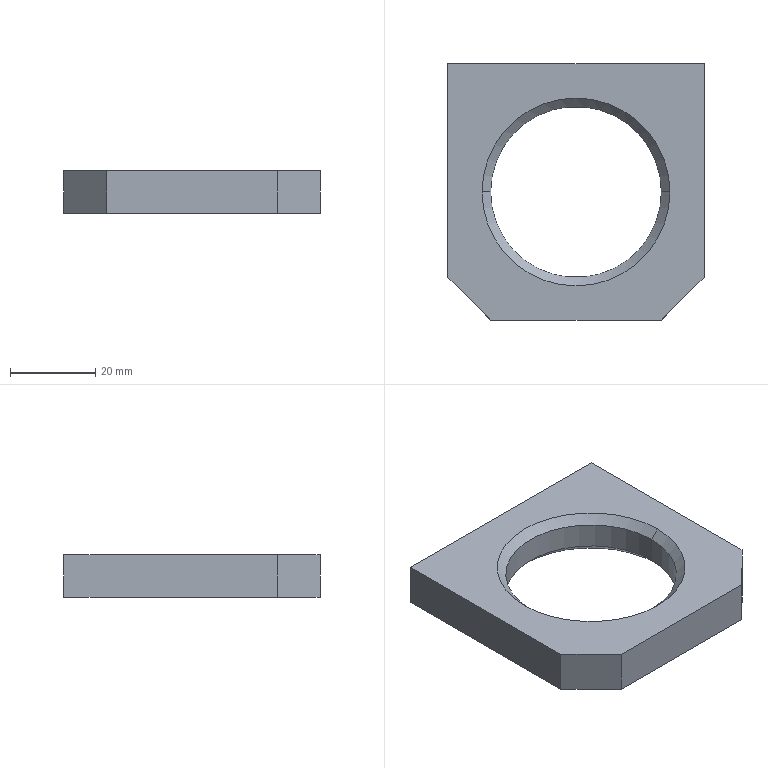Part | SolidWorks | features Chamfer 2, Extrusion 1 | 1 solid | 14 faces | box 60 x 60 x 10 mm | volume 21914 mm3 | plane 8 | cone 4 | cylinder 2 | commonest cylinder face diameters 40 x2
STEP:
#1=CARTESIAN_POINT('',(-20.,0.,8.));
#2=VERTEX_POINT('',#1);
#3=CARTESIAN_POINT('',(20.,0.,8.));
#4=VERTEX_POINT('',#3);
#5=CARTESIAN_POINT('',(0.,0.,8.));
#6=DIRECTION('',(0.,0.,1.));
#7=DIRECTION('',(-1.,0.,0.));
#8=AXIS2_PLACEMENT_3D('',#5,#6,#7);
#9=CIRCLE('',#8,20.);
#10=EDGE_CURVE('',#2,#4,#9,.T.);
#11=ORIENTED_EDGE('',*,*,#10,.F.);
#12=CARTESIAN_POINT('',(-22.,0.,10.));
#13=VERTEX_POINT('',#12);
#14=CARTESIAN_POINT('',(-20.,0.,8.));
#15=DIRECTION('',(-0.7071,0.,0.7071));
#16=VECTOR('',#15,1000.);
#17=LINE('',#14,#16);
#18=EDGE_CURVE('',#2,#13,#17,.T.);
#19=ORIENTED_EDGE('',*,*,#18,.T.);
#20=CARTESIAN_POINT('',(22.,0.,10.));
#21=VERTEX_POINT('',#20);
#22=CARTESIAN_POINT('',(0.,0.,10.));
#23=DIRECTION('',(0.,0.,-1.));
#24=DIRECTION('',(-1.,0.,0.));
#25=AXIS2_PLACEMENT_3D('',#22,#23,#24);
#26=CIRCLE('',#25,22.);
#27=EDGE_CURVE('',#21,#13,#26,.T.);
#28=ORIENTED_EDGE('',*,*,#27,.F.);
#29=CARTESIAN_POINT('',(20.,0.,8.));
#30=DIRECTION('',(0.7071,0.,0.7071));
#31=VECTOR('',#30,1000.);
#32=LINE('',#29,#31);
#33=EDGE_CURVE('',#4,#21,#32,.T.);
#34=ORIENTED_EDGE('',*,*,#33,.F.);
#35=EDGE_LOOP('',(#11,#19,#28,#34));
#36=FACE_OUTER_BOUND('',#35,.T.);
#37=CARTESIAN_POINT('',(0.,0.,8.));
#38=DIRECTION('',(0.,0.,1.));
#39=DIRECTION('',(1.,0.,0.));
#40=AXIS2_PLACEMENT_3D('',#37,#38,#39);
#41=CONICAL_SURFACE('',#40,20.,0.7854);
#42=ADVANCED_FACE('',(#36),#41,.F.);
#43=CARTESIAN_POINT('',(20.,0.,2.));
#44=VERTEX_POINT('',#43);
#45=CARTESIAN_POINT('',(-20.,0.,2.));
#46=VERTEX_POINT('',#45);
#47=CARTESIAN_POINT('',(0.,0.,2.));
#48=DIRECTION('',(0.,0.,-1.));
#49=DIRECTION('',(-1.,0.,0.));
#50=AXIS2_PLACEMENT_3D('',#47,#48,#49);
#51=CIRCLE('',#50,20.);
#52=EDGE_CURVE('',#44,#46,#51,.T.);
#53=ORIENTED_EDGE('',*,*,#52,.F.);
#54=CARTESIAN_POINT('',(22.,0.,0.));
#55=VERTEX_POINT('',#54);
#56=CARTESIAN_POINT('',(22.,0.,0.));
#57=DIRECTION('',(0.7071,0.,-0.7071));
#58=VECTOR('',#57,1000.);
#59=LINE('',#56,#58);
#60=EDGE_CURVE('',#44,#55,#59,.T.);
#61=ORIENTED_EDGE('',*,*,#60,.T.);
#62=CARTESIAN_POINT('',(-22.,0.,0.));
#63=VERTEX_POINT('',#62);
#64=CARTESIAN_POINT('',(0.,0.,0.));
#65=DIRECTION('',(0.,0.,1.));
#66=DIRECTION('',(-1.,0.,0.));
#67=AXIS2_PLACEMENT_3D('',#64,#65,#66);
#68=CIRCLE('',#67,22.);
#69=EDGE_CURVE('',#63,#55,#68,.T.);
#70=ORIENTED_EDGE('',*,*,#69,.F.);
#71=CARTESIAN_POINT('',(-22.,0.,0.));
#72=DIRECTION('',(-0.7071,0.,-0.7071));
#73=VECTOR('',#72,1000.);
#74=LINE('',#71,#73);
#75=EDGE_CURVE('',#46,#63,#74,.T.);
#76=ORIENTED_EDGE('',*,*,#75,.F.);
#77=EDGE_LOOP('',(#53,#61,#70,#76));
#78=FACE_OUTER_BOUND('',#77,.T.);
#79=CARTESIAN_POINT('',(0.,0.,0.));
#80=DIRECTION('',(0.,0.,-1.));
#81=DIRECTION('',(-1.,0.,0.));
#82=AXIS2_PLACEMENT_3D('',#79,#80,#81);
#83=CONICAL_SURFACE('',#82,22.,0.7854);
#84=ADVANCED_FACE('',(#78),#83,.F.);
#85=ORIENTED_EDGE('',*,*,#10,.T.);
#86=CARTESIAN_POINT('',(20.,0.,10.));
#87=DIRECTION('',(0.,0.,-1.));
#88=VECTOR('',#87,1000.);
#89=LINE('',#86,#88);
#90=EDGE_CURVE('',#4,#44,#89,.T.);
#91=ORIENTED_EDGE('',*,*,#90,.T.);
#92=ORIENTED_EDGE('',*,*,#52,.T.);
#93=CARTESIAN_POINT('',(-20.,0.,10.));
#94=DIRECTION('',(0.,0.,-1.));
#95=VECTOR('',#94,1000.);
#96=LINE('',#93,#95);
#97=EDGE_CURVE('',#2,#46,#96,.T.);
#98=ORIENTED_EDGE('',*,*,#97,.F.);
#99=EDGE_LOOP('',(#85,#91,#92,#98));
#100=FACE_OUTER_BOUND('',#99,.T.);
#101=CARTESIAN_POINT('',(0.,0.,10.));
#102=DIRECTION('',(0.,0.,-1.));
#103=DIRECTION('',(-1.,0.,0.));
#104=AXIS2_PLACEMENT_3D('',#101,#102,#103);
#105=CYLINDRICAL_SURFACE('',#104,20.);
#106=ADVANCED_FACE('',(#100),#105,.F.);
#107=ORIENTED_EDGE('',*,*,#27,.T.);
#108=CARTESIAN_POINT('',(0.,0.,10.));
#109=DIRECTION('',(0.,0.,-1.));
#110=DIRECTION('',(-1.,0.,0.));
#111=AXIS2_PLACEMENT_3D('',#108,#109,#110);
#112=CIRCLE('',#111,22.);
#113=EDGE_CURVE('',#13,#21,#112,.T.);
#114=ORIENTED_EDGE('',*,*,#113,.T.);
#115=EDGE_LOOP('',(#107,#114));
#116=FACE_BOUND('',#115,.T.);
#117=CARTESIAN_POINT('',(-20.,-30.,10.));
#118=VERTEX_POINT('',#117);
#119=CARTESIAN_POINT('',(20.,-30.,10.));
#120=VERTEX_POINT('',#119);
#121=CARTESIAN_POINT('',(-30.,-30.,10.));
#122=DIRECTION('',(1.,0.,0.));
#123=VECTOR('',#122,1000.);
#124=LINE('',#121,#123);
#125=EDGE_CURVE('',#118,#120,#124,.T.);
#126=ORIENTED_EDGE('',*,*,#125,.T.);
#127=CARTESIAN_POINT('',(30.,-20.,10.));
#128=VERTEX_POINT('',#127);
#129=CARTESIAN_POINT('',(30.,-20.,10.));
#130=DIRECTION('',(0.7071,0.7071,0.));
#131=VECTOR('',#130,1000.);
#132=LINE('',#129,#131);
#133=EDGE_CURVE('',#120,#128,#132,.T.);
#134=ORIENTED_EDGE('',*,*,#133,.T.);
#135=CARTESIAN_POINT('',(30.,30.,10.));
#136=VERTEX_POINT('',#135);
#137=CARTESIAN_POINT('',(30.,-30.,10.));
#138=DIRECTION('',(0.,1.,0.));
#139=VECTOR('',#138,1000.);
#140=LINE('',#137,#139);
#141=EDGE_CURVE('',#128,#136,#140,.T.);
#142=ORIENTED_EDGE('',*,*,#141,.T.);
#143=CARTESIAN_POINT('',(-30.,30.,10.));
#144=VERTEX_POINT('',#143);
#145=CARTESIAN_POINT('',(-30.,30.,10.));
#146=DIRECTION('',(-1.,0.,0.));
#147=VECTOR('',#146,1000.);
#148=LINE('',#145,#147);
#149=EDGE_CURVE('',#136,#144,#148,.T.);
#150=ORIENTED_EDGE('',*,*,#149,.T.);
#151=CARTESIAN_POINT('',(-30.,-20.,10.));
#152=VERTEX_POINT('',#151);
#153=CARTESIAN_POINT('',(-30.,-30.,10.));
#154=DIRECTION('',(0.,-1.,0.));
#155=VECTOR('',#154,1000.);
#156=LINE('',#153,#155);
#157=EDGE_CURVE('',#144,#152,#156,.T.);
#158=ORIENTED_EDGE('',*,*,#157,.T.);
#159=CARTESIAN_POINT('',(-20.,-30.,10.));
#160=DIRECTION('',(0.7071,-0.7071,0.));
#161=VECTOR('',#160,1000.);
#162=LINE('',#159,#161);
#163=EDGE_CURVE('',#152,#118,#162,.T.);
#164=ORIENTED_EDGE('',*,*,#163,.T.);
#165=EDGE_LOOP('',(#126,#134,#142,#150,#158,#164));
#166=FACE_OUTER_BOUND('',#165,.T.);
#167=CARTESIAN_POINT('',(0.,0.,10.));
#168=DIRECTION('',(0.,0.,-1.));
#169=DIRECTION('',(-1.,0.,0.));
#170=AXIS2_PLACEMENT_3D('',#167,#168,#169);
#171=PLANE('',#170);
#172=ADVANCED_FACE('',(#116,#166),#171,.F.);
#173=ORIENTED_EDGE('',*,*,#69,.T.);
#174=CARTESIAN_POINT('',(0.,0.,0.));
#175=DIRECTION('',(0.,0.,1.));
#176=DIRECTION('',(-1.,0.,0.));
#177=AXIS2_PLACEMENT_3D('',#174,#175,#176);
#178=CIRCLE('',#177,22.);
#179=EDGE_CURVE('',#55,#63,#178,.T.);
#180=ORIENTED_EDGE('',*,*,#179,.T.);
#181=EDGE_LOOP('',(#173,#180));
#182=FACE_BOUND('',#181,.T.);
#183=CARTESIAN_POINT('',(30.,-20.,0.));
#184=VERTEX_POINT('',#183);
#185=CARTESIAN_POINT('',(30.,30.,0.));
#186=VERTEX_POINT('',#185);
#187=CARTESIAN_POINT('',(30.,-30.,0.));
#188=DIRECTION('',(0.,1.,0.));
#189=VECTOR('',#188,1000.);
#190=LINE('',#187,#189);
#191=EDGE_CURVE('',#184,#186,#190,.T.);
#192=ORIENTED_EDGE('',*,*,#191,.F.);
#193=CARTESIAN_POINT('',(20.,-30.,0.));
#194=VERTEX_POINT('',#193);
#195=CARTESIAN_POINT('',(25.,-25.,0.));
#196=DIRECTION('',(-0.7071,-0.7071,0.));
#197=VECTOR('',#196,1000.);
#198=LINE('',#195,#197);
#199=EDGE_CURVE('',#184,#194,#198,.T.);
#200=ORIENTED_EDGE('',*,*,#199,.T.);
#201=CARTESIAN_POINT('',(-20.,-30.,0.));
#202=VERTEX_POINT('',#201);
#203=CARTESIAN_POINT('',(-30.,-30.,0.));
#204=DIRECTION('',(1.,0.,0.));
#205=VECTOR('',#204,1000.);
#206=LINE('',#203,#205);
#207=EDGE_CURVE('',#202,#194,#206,.T.);
#208=ORIENTED_EDGE('',*,*,#207,.F.);
#209=CARTESIAN_POINT('',(-30.,-20.,0.));
#210=VERTEX_POINT('',#209);
#211=CARTESIAN_POINT('',(-25.,-25.,0.));
#212=DIRECTION('',(-0.7071,0.7071,0.));
#213=VECTOR('',#212,1000.);
#214=LINE('',#211,#213);
#215=EDGE_CURVE('',#202,#210,#214,.T.);
#216=ORIENTED_EDGE('',*,*,#215,.T.);
#217=CARTESIAN_POINT('',(-30.,30.,0.));
#218=VERTEX_POINT('',#217);
#219=CARTESIAN_POINT('',(-30.,-30.,0.));
#220=DIRECTION('',(0.,-1.,0.));
#221=VECTOR('',#220,1000.);
#222=LINE('',#219,#221);
#223=EDGE_CURVE('',#218,#210,#222,.T.);
#224=ORIENTED_EDGE('',*,*,#223,.F.);
#225=CARTESIAN_POINT('',(-30.,30.,0.));
#226=DIRECTION('',(-1.,0.,0.));
#227=VECTOR('',#226,1000.);
#228=LINE('',#225,#227);
#229=EDGE_CURVE('',#186,#218,#228,.T.);
#230=ORIENTED_EDGE('',*,*,#229,.F.);
#231=EDGE_LOOP('',(#192,#200,#208,#216,#224,#230));
#232=FACE_OUTER_BOUND('',#231,.T.);
#233=CARTESIAN_POINT('',(0.,0.,0.));
#234=DIRECTION('',(0.,0.,-1.));
#235=DIRECTION('',(-1.,0.,0.));
#236=AXIS2_PLACEMENT_3D('',#233,#234,#235);
#237=PLANE('',#236);
#238=ADVANCED_FACE('',(#182,#232),#237,.T.);
#239=ORIENTED_EDGE('',*,*,#141,.F.);
#240=CARTESIAN_POINT('',(30.,-20.,10.));
#241=DIRECTION('',(0.,0.,-1.));
#242=VECTOR('',#241,1000.);
#243=LINE('',#240,#242);
#244=EDGE_CURVE('',#128,#184,#243,.T.);
#245=ORIENTED_EDGE('',*,*,#244,.T.);
#246=ORIENTED_EDGE('',*,*,#191,.T.);
#247=CARTESIAN_POINT('',(30.,30.,10.));
#248=DIRECTION('',(0.,0.,-1.));
#249=VECTOR('',#248,1000.);
#250=LINE('',#247,#249);
#251=EDGE_CURVE('',#136,#186,#250,.T.);
#252=ORIENTED_EDGE('',*,*,#251,.F.);
#253=EDGE_LOOP('',(#239,#245,#246,#252));
#254=FACE_OUTER_BOUND('',#253,.T.);
#255=CARTESIAN_POINT('',(30.,-30.,10.));
#256=DIRECTION('',(-1.,0.,0.));
#257=DIRECTION('',(0.,0.,1.));
#258=AXIS2_PLACEMENT_3D('',#255,#256,#257);
#259=PLANE('',#258);
#260=ADVANCED_FACE('',(#254),#259,.F.);
#261=ORIENTED_EDGE('',*,*,#229,.T.);
#262=CARTESIAN_POINT('',(-30.,30.,10.));
#263=DIRECTION('',(0.,0.,-1.));
#264=VECTOR('',#263,1000.);
#265=LINE('',#262,#264);
#266=EDGE_CURVE('',#144,#218,#265,.T.);
#267=ORIENTED_EDGE('',*,*,#266,.F.);
#268=ORIENTED_EDGE('',*,*,#149,.F.);
#269=ORIENTED_EDGE('',*,*,#251,.T.);
#270=EDGE_LOOP('',(#261,#267,#268,#269));
#271=FACE_OUTER_BOUND('',#270,.T.);
#272=CARTESIAN_POINT('',(-30.,30.,10.));
#273=DIRECTION('',(0.,-1.,0.));
#274=DIRECTION('',(0.,0.,-1.));
#275=AXIS2_PLACEMENT_3D('',#272,#273,#274);
#276=PLANE('',#275);
#277=ADVANCED_FACE('',(#271),#276,.F.);
#278=ORIENTED_EDGE('',*,*,#223,.T.);
#279=CARTESIAN_POINT('',(-30.,-20.,10.));
#280=DIRECTION('',(0.,0.,1.));
#281=VECTOR('',#280,1000.);
#282=LINE('',#279,#281);
#283=EDGE_CURVE('',#210,#152,#282,.T.);
#284=ORIENTED_EDGE('',*,*,#283,.T.);
#285=ORIENTED_EDGE('',*,*,#157,.F.);
#286=ORIENTED_EDGE('',*,*,#266,.T.);
#287=EDGE_LOOP('',(#278,#284,#285,#286));
#288=FACE_OUTER_BOUND('',#287,.T.);
#289=CARTESIAN_POINT('',(-30.,-30.,10.));
#290=DIRECTION('',(1.,0.,0.));
#291=DIRECTION('',(0.,0.,-1.));
#292=AXIS2_PLACEMENT_3D('',#289,#290,#291);
#293=PLANE('',#292);
#294=ADVANCED_FACE('',(#288),#293,.F.);
#295=ORIENTED_EDGE('',*,*,#207,.T.);
#296=CARTESIAN_POINT('',(20.,-30.,10.));
#297=DIRECTION('',(0.,0.,1.));
#298=VECTOR('',#297,1000.);
#299=LINE('',#296,#298);
#300=EDGE_CURVE('',#194,#120,#299,.T.);
#301=ORIENTED_EDGE('',*,*,#300,.T.);
#302=ORIENTED_EDGE('',*,*,#125,.F.);
#303=CARTESIAN_POINT('',(-20.,-30.,10.));
#304=DIRECTION('',(0.,0.,-1.));
#305=VECTOR('',#304,1000.);
#306=LINE('',#303,#305);
#307=EDGE_CURVE('',#118,#202,#306,.T.);
#308=ORIENTED_EDGE('',*,*,#307,.T.);
#309=EDGE_LOOP('',(#295,#301,#302,#308));
#310=FACE_OUTER_BOUND('',#309,.T.);
#311=CARTESIAN_POINT('',(-30.,-30.,10.));
#312=DIRECTION('',(0.,1.,0.));
#313=DIRECTION('',(0.,0.,1.));
#314=AXIS2_PLACEMENT_3D('',#311,#312,#313);
#315=PLANE('',#314);
#316=ADVANCED_FACE('',(#310),#315,.F.);
#317=ORIENTED_EDGE('',*,*,#90,.F.);
#318=CARTESIAN_POINT('',(0.,0.,8.));
#319=DIRECTION('',(0.,0.,1.));
#320=DIRECTION('',(-1.,0.,0.));
#321=AXIS2_PLACEMENT_3D('',#318,#319,#320);
#322=CIRCLE('',#321,20.);
#323=EDGE_CURVE('',#4,#2,#322,.T.);
#324=ORIENTED_EDGE('',*,*,#323,.T.);
#325=ORIENTED_EDGE('',*,*,#97,.T.);
#326=CARTESIAN_POINT('',(0.,0.,2.));
#327=DIRECTION('',(0.,0.,-1.));
#328=DIRECTION('',(-1.,0.,0.));
#329=AXIS2_PLACEMENT_3D('',#326,#327,#328);
#330=CIRCLE('',#329,20.);
#331=EDGE_CURVE('',#46,#44,#330,.T.);
#332=ORIENTED_EDGE('',*,*,#331,.T.);
#333=EDGE_LOOP('',(#317,#324,#325,#332));
#334=FACE_OUTER_BOUND('',#333,.T.);
#335=CARTESIAN_POINT('',(0.,0.,10.));
#336=DIRECTION('',(0.,0.,-1.));
#337=DIRECTION('',(-1.,0.,0.));
#338=AXIS2_PLACEMENT_3D('',#335,#336,#337);
#339=CYLINDRICAL_SURFACE('',#338,20.);
#340=ADVANCED_FACE('',(#334),#339,.F.);
#341=ORIENTED_EDGE('',*,*,#133,.F.);
#342=ORIENTED_EDGE('',*,*,#300,.F.);
#343=ORIENTED_EDGE('',*,*,#199,.F.);
#344=ORIENTED_EDGE('',*,*,#244,.F.);
#345=EDGE_LOOP('',(#341,#342,#343,#344));
#346=FACE_OUTER_BOUND('',#345,.T.);
#347=CARTESIAN_POINT('',(30.,-20.,10.));
#348=DIRECTION('',(-0.7071,0.7071,0.));
#349=DIRECTION('',(0.,0.,-1.));
#350=AXIS2_PLACEMENT_3D('',#347,#348,#349);
#351=PLANE('',#350);
#352=ADVANCED_FACE('',(#346),#351,.F.);
#353=ORIENTED_EDGE('',*,*,#163,.F.);
#354=ORIENTED_EDGE('',*,*,#283,.F.);
#355=ORIENTED_EDGE('',*,*,#215,.F.);
#356=ORIENTED_EDGE('',*,*,#307,.F.);
#357=EDGE_LOOP('',(#353,#354,#355,#356));
#358=FACE_OUTER_BOUND('',#357,.T.);
#359=CARTESIAN_POINT('',(-20.,-30.,10.));
#360=DIRECTION('',(0.7071,0.7071,0.));
#361=DIRECTION('',(0.,0.,-1.));
#362=AXIS2_PLACEMENT_3D('',#359,#360,#361);
#363=PLANE('',#362);
#364=ADVANCED_FACE('',(#358),#363,.F.);
#365=ORIENTED_EDGE('',*,*,#60,.F.);
#366=ORIENTED_EDGE('',*,*,#331,.F.);
#367=ORIENTED_EDGE('',*,*,#75,.T.);
#368=ORIENTED_EDGE('',*,*,#179,.F.);
#369=EDGE_LOOP('',(#365,#366,#367,#368));
#370=FACE_OUTER_BOUND('',#369,.T.);
#371=CARTESIAN_POINT('',(0.,0.,0.));
#372=DIRECTION('',(0.,0.,-1.));
#373=DIRECTION('',(-1.,0.,0.));
#374=AXIS2_PLACEMENT_3D('',#371,#372,#373);
#375=CONICAL_SURFACE('',#374,22.,0.7854);
#376=ADVANCED_FACE('',(#370),#375,.F.);
#377=ORIENTED_EDGE('',*,*,#18,.F.);
#378=ORIENTED_EDGE('',*,*,#323,.F.);
#379=ORIENTED_EDGE('',*,*,#33,.T.);
#380=ORIENTED_EDGE('',*,*,#113,.F.);
#381=EDGE_LOOP('',(#377,#378,#379,#380));
#382=FACE_OUTER_BOUND('',#381,.T.);
#383=CARTESIAN_POINT('',(0.,0.,8.));
#384=DIRECTION('',(0.,0.,1.));
#385=DIRECTION('',(1.,0.,0.));
#386=AXIS2_PLACEMENT_3D('',#383,#384,#385);
#387=CONICAL_SURFACE('',#386,20.,0.7854);
#388=ADVANCED_FACE('',(#382),#387,.F.);
#389=CLOSED_SHELL('',(#42,#84,#106,#172,#238,#260,#277,#294,#316,#340,#352,#364,#376,#388));
#390=MANIFOLD_SOLID_BREP('',#389);
#391=CARTESIAN_POINT('',(0.,0.,0.));
#392=DIRECTION('',(0.,0.,1.));
#393=DIRECTION('',(1.,0.,0.));
#394=AXIS2_PLACEMENT_3D('',#391,#392,#393);
#395=(LENGTH_UNIT()NAMED_UNIT(*)SI_UNIT(.MILLI.,.METRE.));
#396=UNCERTAINTY_MEASURE_WITH_UNIT(LENGTH_MEASURE(0.00001),#395,'','');
#397=(NAMED_UNIT(*)PLANE_ANGLE_UNIT()SI_UNIT($,.RADIAN.));
#398=(NAMED_UNIT(*)SI_UNIT($,.STERADIAN.)SOLID_ANGLE_UNIT());
#399=(GEOMETRIC_REPRESENTATION_CONTEXT(3)GLOBAL_UNCERTAINTY_ASSIGNED_CONTEXT((#396))GLOBAL_UNIT_ASSIGNED_CONTEXT((#395,#397,#398))REPRESENTATION_CONTEXT('',''));
#400=ADVANCED_BREP_SHAPE_REPRESENTATION('',(#390,#394),#399);